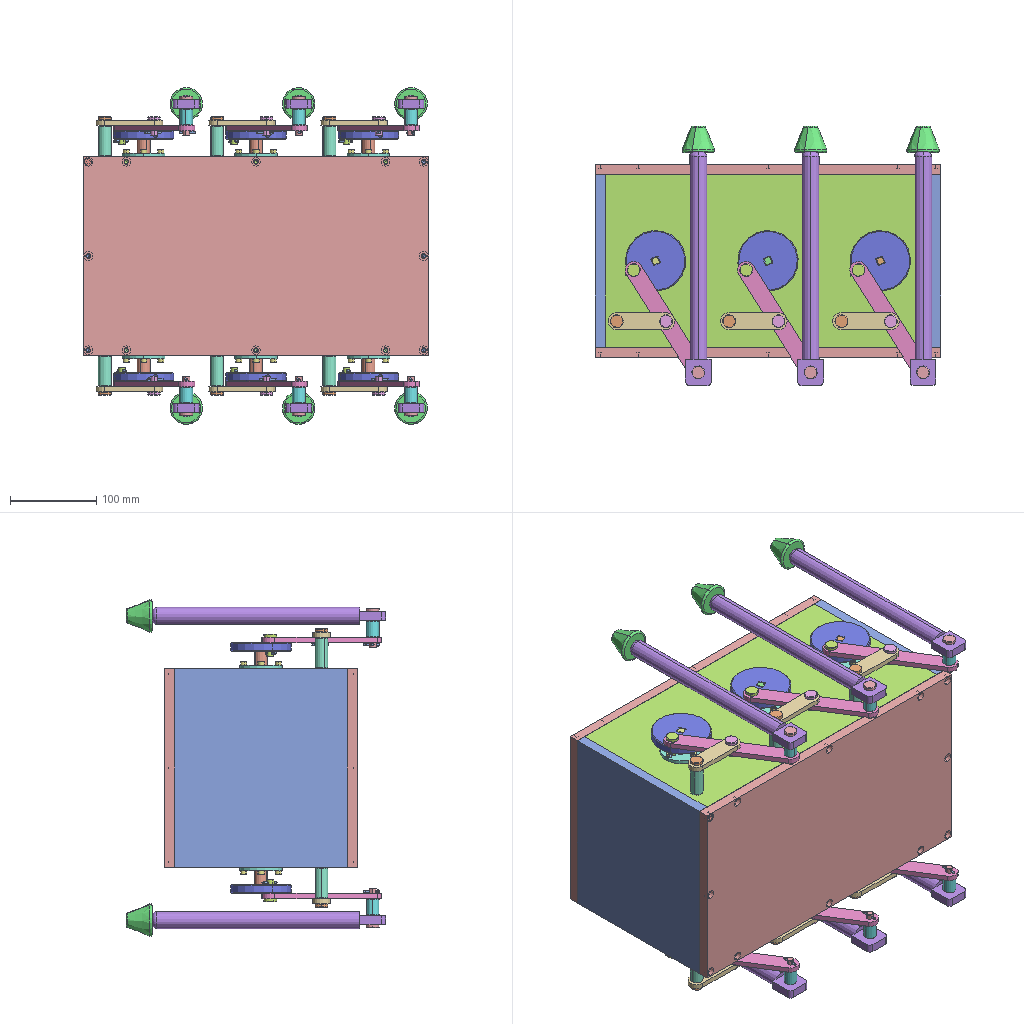Assembly | SolidWorks | 34 different items | 170 placed | box 400 x 300 x 390 mm
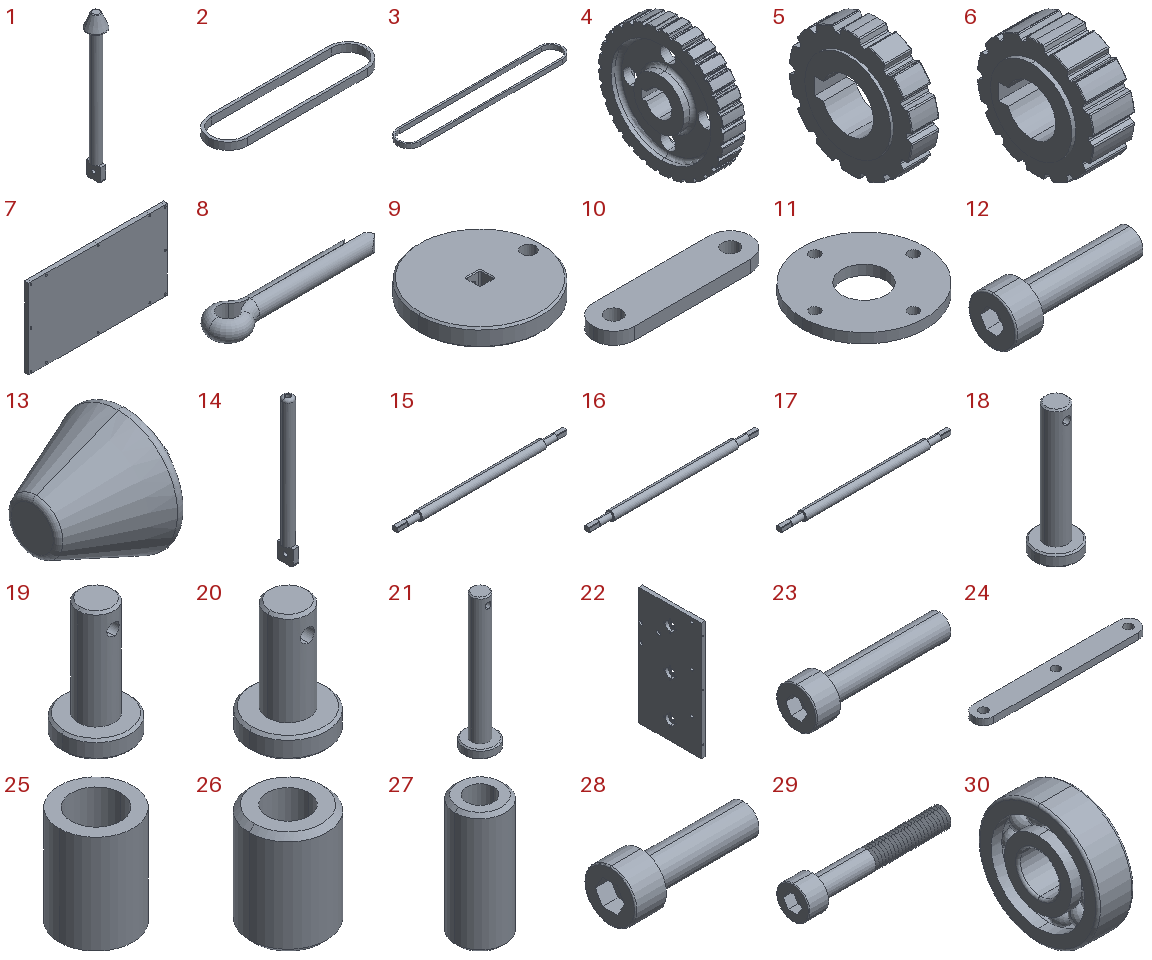Parts list (item | name | quantity | parent item | size | volume | features):
1 | (subassembly) | x6 | - | 38.092 x 38.092 x 300 mm | 102334 mm3 | -
2 | - | x1 | - | 171.8 x 41.8 x 7.9 mm | 9051 mm3 | features Extrusion 1, Shell 1
3 | - | x1 | - | 301.8 x 41.8 x 7.9 mm | 15213 mm3 | features Extrusion 1, Shell 1
4 | - | x1 | - | 15.24 x 72.254 x 72.292 mm | 33206 mm3 | features Cut 3, CirPattern 2, ICE 2, Chamfer 1, Fillet 1, RefAxis 1, Revolution 1
5 | - | x4 | - | 9.48 x 35.738 x 35.892 mm | 6598 mm3 | features ICE 3, Cut 2, Chamfer 1, CirPattern 1, Fillet 1, RefAxis 1, Revolution 1
6 | - | x1 | - | 15.24 x 35.738 x 35.892 mm | 10593 mm3 | features ICE 3, Cut 2, Chamfer 1, CirPattern 1, Fillet 1, RefAxis 1, Revolution 1
7 | - | x2 | - | 400 x 12 x 230 mm | 1097029 mm3 | features Extrusion 1, HoleWzd 1
8 | - | x24 | - | 19.5 x 4.6 x 2.3 mm | 75.866 mm3 | features ICE 1, Sweep 1
9 | - | x6 | - | 70 x 70 x 10 mm | 36483 mm3 | features ICE 4, Chamfer 2, 3DProfileFeature 1, Cut 1, Extrusion 1, Fillet 1, HoleWzd 1
10 | - | x6 | - | 77.02 x 20 x 6 mm | 8124 mm3 | features Extrusion 1, ICE 1
11 | - | x6 | - | 50 x 50 x 4 mm | 6614 mm3 | features Extrusion 1
12 | - | x24 | - | 20 x 7 x 7 mm | 339.552 mm3 | features BlendCut 1, Cut 1, Fillet 1, LPattern 1, RevCut 1, Revolution 1
13 | - | x6 | in 1 | 40 x 38.092 x 38.092 mm | 19850 mm3 | features Fillet 2, ICE 1, Revolution 1
14 | - | x6 | in 1 | 20 x 30 x 270 mm | 82484 mm3 | features ICE 3, Fillet 2, Extrusion 1
15 | - | x1 | - | 290 x 17.22 x 15 mm | 43056 mm3 | features ICE 3, Chamfer 1, Cut 1, Extrusion 1, Fillet 1, MirrorPattern 1
16 | - | x1 | - | 290 x 17.22 x 15 mm | 43172 mm3 | features ICE 3, Chamfer 1, Cut 1, Extrusion 1, Fillet 1, MirrorPattern 1
17 | - | x1 | - | 290 x 15 x 17.22 mm | 43129 mm3 | features ICE 3, Chamfer 1, Cut 1, Extrusion 1, Fillet 1, MirrorPattern 1
18 | - | x6 | - | 15 x 15 x 46 mm | 2758 mm3 | features ICE 2, Chamfer 1, Extrusion 1
19 | - | x6 | - | 15 x 15 x 26 mm | 1753 mm3 | features ICE 2, Chamfer 1, Extrusion 1
20 | - | x6 | - | 15 x 15 x 22 mm | 1552 mm3 | features ICE 2, Chamfer 1, Extrusion 1
21 | - | x6 | - | 15 x 15 x 64 mm | 3663 mm3 | features ICE 2, Chamfer 1, Extrusion 1
22 | - | x1 | - | 12 x 200 x 376 mm | 873388 mm3 | features HoleWzd 1, MirrorStock 1
23 | - | x2 | - | 30 x 8.5 x 8.5 mm | 740.448 mm3 | features BlendCut 1, Cut 1, Fillet 1, LPattern 1, RevCut 1, Revolution 1
24 | - | x6 | - | 160 x 20 x 6 mm | 17780 mm3 | features ICE 2, Extrusion 1
25 | - | x6 | - | 15 x 15 x 20 mm | 1963 mm3 | features Extrusion 1
26 | - | x6 | - | 15 x 15 x 20 mm | 2484 mm3 | features Chamfer 1, Extrusion 1, ICE 1
27 | - | x6 | - | 15 x 15 x 36 mm | 4507 mm3 | features Chamfer 1, Extrusion 1, ICE 1
28 | - | x3 | - | 26 x 10 x 10 mm | 972.813 mm3 | features BlendCut 1, Cut 1, Fillet 1, LPattern 1, RevCut 1, Revolution 1
29 | - | x3 | - | 46 x 10 x 10 mm | 1365 mm3 | features BlendCut 1, Cut 1, Fillet 1, LPattern 1, RevCut 1, Revolution 1
30 | - | x6 | - | 9 x 30 x 30 mm | 4205 mm3 | features Revolution 3, CirPattern 1, Fillet 1
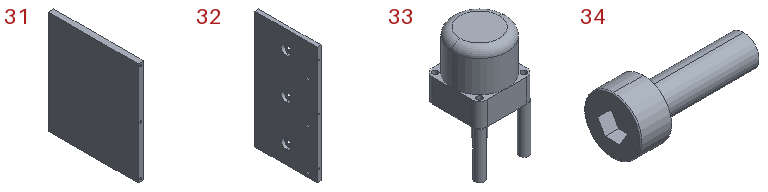31 | - | x2 | - | 12 x 200 x 230 mm | 549928 mm3 | features Extrusion 1, HoleWzd 1, MirrorPattern 1
32 | - | x1 | - | 12 x 200 x 376 mm | 876393 mm3 | features Cut 2, HoleWzd 2, Extrusion 1, ICE 1, MirrorPattern 1
33 | - | x1 | - | 70 x 70 x 140 mm | 361948 mm3 | features Chamfer 5, ICE 5, Fillet 2, HoleWzd 2, CirPattern 1, Extrusion 1
34 | - | x6 | - | 13 x 5.5 x 5.5 mm | 134.528 mm3 | features BlendCut 1, Cut 1, Fillet 1, LPattern 1, RevCut 1, Revolution 1
Mates (type | each side: item.copy, entity, surface, feature):
In the top assembly
Concentric | 7.1 face cylinder CBORE for M5 Hex Socket Head Cap Screw1 | 31.1 face cylinder M5 Tapped Hole1 | 2 times
Coincident | 7.1 face plane Boss-Extrude1 | 31.1 face plane Boss-Extrude1
Concentric | 7.1 face cylinder CBORE for M5 Hex Socket Head Cap Screw1 | 31.2 edge
Concentric | 7.1 face cylinder CBORE for M5 Hex Socket Head Cap Screw1 | 31.2 face cylinder M5 Tapped Hole1
Coincident | 7.1 face plane Boss-Extrude1 | 31.2 face plane Boss-Extrude1
Concentric | 7.1 face cylinder CBORE for M5 Hex Socket Head Cap Screw1 | 32.1 face cylinder Mirror1 | 2 times
Coincident | 7.1 face plane Boss-Extrude1 | 32.1 face plane Boss-Extrude1
Concentric | 31.1 face cylinder Mirror1 | 7.2 face cylinder CBORE for M5 Hex Socket Head Cap Screw1
Concentric | 32.1 face cylinder Mirror1 | 7.2 face cylinder CBORE for M5 Hex Socket Head Cap Screw1
Coincident | 31.1 face plane Boss-Extrude1 | 7.2 face plane Boss-Extrude1
Concentric | 32.1 face cylinder Cut-Extrude1 | 30.1 face cylinder Revolve3
Coincident | 32.1 face plane Boss-Extrude1 | 30.1 face plane Revolve3
Concentric | 32.1 face cylinder Cut-Extrude1 | 30.2 face cylinder Revolve3
Coincident | 32.1 face plane Boss-Extrude1 | 30.2 face plane Revolve3
Concentric | 32.1 face cylinder Cut-Extrude1 | 30.3 face cylinder Revolve3
Coincident | 32.1 face plane Boss-Extrude1 | 30.3 face plane Revolve3
Concentric | 30.4 face cylinder Revolve2 | 11.1 face cylinder Boss-Extrude1
Concentric | 30.3 face cylinder Revolve2 | 11.2 face cylinder Boss-Extrude1
Coincident | 32.1 face plane Boss-Extrude1 | 11.2 face plane Boss-Extrude1
Concentric | 30.1 face cylinder Revolve2 | 15.1 face cylinder Boss-Extrude1
Coincident | 30.1 face plane Revolve2 | 15.1 face plane Boss-Extrude1
Concentric | 30.2 face cylinder Revolve2 | 16.1 face cylinder Boss-Extrude1
Coincident | 30.2 face plane Revolve2 | 16.1 face plane Boss-Extrude1
Concentric | 30.3 face cylinder Revolve2 | 17.1 face cylinder Boss-Extrude1
Coincident | 30.3 face plane Revolve2 | 17.1 face plane Boss-Extrude1
Concentric | 17.1 face cylinder Boss-Extrude2 | 25.1 face cylinder Boss-Extrude1
Coincident | 30.4 face plane Revolve2 | 25.1 face plane Boss-Extrude1
Concentric | 17.1 face cylinder Boss-Extrude2 | 25.2 face cylinder Boss-Extrude1
Coincident | 30.3 face plane Revolve2 | 25.2 face plane Boss-Extrude1
Coincident | 17.1 face plane Cut-Extrude1 | 9.1 face plane Cut-Extrude3 | 2 times
Coincident | 25.1 face plane Boss-Extrude1 | 9.1 face plane Boss-Extrude1
Coincident | 16.1 face plane Mirror1 | 9.2 face plane Cut-Extrude3 | 2 times
Coincident | 25.3 face plane Boss-Extrude1 | 9.2 face plane Boss-Extrude1
Coincident | 15.1 face plane Cut-Extrude1 | 9.3 face plane Cut-Extrude3 | 2 times
Coincident | 25.4 face plane Boss-Extrude1 | 9.3 face plane Boss-Extrude1
Coincident | 17.1 face plane Mirror1 | 9.4 face plane Cut-Extrude3 | 2 times
Coincident | 25.2 face plane Boss-Extrude1 | 9.4 face plane Boss-Extrude1
Coincident | 16.1 face plane Cut-Extrude1 | 9.5 face plane Cut-Extrude3 | 2 times
Coincident | 25.5 face plane Boss-Extrude1 | 9.5 face plane Boss-Extrude1
Coincident | 15.1 face plane Mirror1 | 9.6 face plane Cut-Extrude3 | 2 times
Coincident | 25.6 face plane Boss-Extrude1 | 9.6 face plane Boss-Extrude1
Concentric | 9.6 face cylinder Cut-Extrude2 | 24.1 face cylinder Cut-Extrude1
Coincident | 9.6 face plane Boss-Extrude1 | 24.1 face plane Boss-Extrude1
Concentric | 9.5 face cylinder Cut-Extrude2 | 24.2 face cylinder Cut-Extrude1
Coincident | 9.5 face plane Boss-Extrude1 | 24.2 face plane Boss-Extrude1
Concentric | 9.4 face cylinder Cut-Extrude2 | 24.3 face cylinder Cut-Extrude1
Coincident | 9.4 face plane Boss-Extrude1 | 24.3 face plane Boss-Extrude1
Concentric | 9.3 face cylinder Cut-Extrude2 | 24.4 face cylinder Cut-Extrude1
Coincident | 9.3 face plane Boss-Extrude1 | 24.4 face plane Boss-Extrude1
Coincident | 9.2 face plane Boss-Extrude1 | 24.5 face plane Boss-Extrude1
Concentric | 9.2 face cylinder Cut-Extrude2 | 24.5 face cylinder Cut-Extrude1
Coincident | 9.1 face plane Boss-Extrude1 | 24.6 face plane Boss-Extrude1
Concentric | 9.1 face cylinder Cut-Extrude2 | 24.6 face cylinder Cut-Extrude1
Coincident | 24.3 face plane Boss-Extrude1 | 26.1 face plane Boss-Extrude1
Concentric | 24.3 face cylinder Cut-Extrude1 | 26.1 face cylinder Boss-Extrude1
Concentric | 24.2 face cylinder Cut-Extrude1 | 26.2 face cylinder Boss-Extrude1
Coincident | 24.2 face plane Boss-Extrude1 | 26.2 face plane Boss-Extrude1
Concentric | 24.1 edge | 26.3 face cylinder Boss-Extrude1
Coincident | 24.1 face plane Boss-Extrude1 | 26.3 face plane Boss-Extrude1
Concentric | 24.4 face cylinder Cut-Extrude1 | 26.4 face cylinder Boss-Extrude1
Coincident | 24.4 face plane Boss-Extrude1 | 26.4 face plane Boss-Extrude1
Concentric | 24.5 face cylinder Cut-Extrude1 | 26.5 face cylinder Boss-Extrude1
Coincident | 24.5 face plane Boss-Extrude1 | 26.5 face plane Boss-Extrude1
Concentric | 24.6 face cylinder Cut-Extrude1 | 26.6 face cylinder Boss-Extrude1
Coincident | 24.6 face plane Boss-Extrude1 | 26.6 face plane Boss-Extrude1
Concentric | 24.1 face cylinder Cut-Extrude2 | 10.1 face cylinder Cut-Extrude1
Coincident | 24.1 face plane Boss-Extrude1 | 10.1 face plane Boss-Extrude1
Coincident | 24.2 face plane Boss-Extrude1 | 10.2 face plane Boss-Extrude1
Concentric | 24.2 face cylinder Cut-Extrude2 | 10.2 face cylinder Cut-Extrude1
Coincident | 24.3 face plane Boss-Extrude1 | 10.3 face plane Boss-Extrude1
Concentric | 24.3 face cylinder Cut-Extrude2 | 10.3 face cylinder Cut-Extrude1
Coincident | 24.5 face plane Boss-Extrude1 | 10.4 face plane Boss-Extrude1
Concentric | 24.5 face cylinder Cut-Extrude2 | 10.4 face cylinder Cut-Extrude1
Coincident | 24.4 face plane Boss-Extrude1 | 10.5 face plane Boss-Extrude1
Concentric | 24.4 face cylinder Cut-Extrude2 | 10.5 face cylinder Cut-Extrude1
Concentric | 26.4 face cylinder Boss-Extrude1 | 14.1 face cylinder Cut-Extrude1
Coincident | 26.4 face plane Boss-Extrude1 | 14.1 face plane Boss-Extrude2
Concentric | 26.5 face cylinder Boss-Extrude1 | 14.2 face cylinder Cut-Extrude1
Coincident | 26.5 face plane Boss-Extrude1 | 14.2 face plane Boss-Extrude2
Concentric | 26.6 face cylinder Boss-Extrude1 | 14.3 face cylinder Cut-Extrude1
Coincident | 26.6 face plane Boss-Extrude1 | 14.3 face plane Boss-Extrude2
Concentric | 32.1 face cylinder Cut-Extrude3 | 10.1 face cylinder Cut-Extrude1
Concentric | 32.1 face cylinder Cut-Extrude3 | 10.2 face cylinder Cut-Extrude1
Concentric | 32.1 face cylinder Cut-Extrude3 | 10.3 face cylinder Cut-Extrude1
Coincident | 24.6 face plane Boss-Extrude1 | 10.6 face plane Boss-Extrude1
Concentric | 24.6 face cylinder Cut-Extrude2 | 10.6 face cylinder Cut-Extrude1
Concentric | 22.1 face cylinder Side Plate2 Mirror | 10.6 face cylinder Cut-Extrude1
Concentric | 22.1 face cylinder Side Plate2 Mirror | 10.4 face cylinder Cut-Extrude1
Concentric | 22.1 face cylinder Side Plate2 Mirror | 10.5 face cylinder Cut-Extrude1
Concentric | 26.3 face cylinder Boss-Extrude1 | 14.4 face cylinder Cut-Extrude1
Coincident | 26.3 face plane Boss-Extrude1 | 14.4 face plane Boss-Extrude2
Concentric | 26.2 face cylinder Boss-Extrude1 | 14.5 face cylinder Cut-Extrude1
Coincident | 26.2 face plane Boss-Extrude1 | 14.5 face plane Boss-Extrude2
Concentric | 26.1 face cylinder Boss-Extrude1 | 14.6 face cylinder Cut-Extrude1
Coincident | 26.1 face plane Boss-Extrude1 | 14.6 face plane Boss-Extrude2
Coincident | 10.3 face plane Boss-Extrude1 | 10.2 face plane Boss-Extrude1
Coincident | 10.2 face plane Boss-Extrude1 | 10.1 face plane Boss-Extrude1
Concentric | 18.1 face cylinder Boss-Extrude1 | 24.4 face cylinder Cut-Extrude1
Coincident | 14.1 face plane Boss-Extrude2 | 18.1 face plane Boss-Extrude2
Concentric | 14.2 face cylinder Cut-Extrude1 | 18.2 face cylinder Boss-Extrude1
Coincident | 14.2 face plane Boss-Extrude2 | 18.2 face plane Boss-Extrude2
Concentric | 14.3 face cylinder Cut-Extrude1 | 18.3 face cylinder Boss-Extrude1
Coincident | 14.3 face plane Boss-Extrude2 | 18.3 face plane Boss-Extrude2
Coincident | 14.4 edge | 18.4 face cylinder Boss-Extrude1
Coincident | 14.4 face plane Boss-Extrude2 | 18.4 face plane Boss-Extrude2
Concentric | 14.5 face cylinder Cut-Extrude1 | 18.5 face cylinder Boss-Extrude1
Coincident | 14.5 face plane Boss-Extrude2 | 18.5 face plane Boss-Extrude2
Coincident | 14.6 edge | 18.6 face cylinder Boss-Extrude1
Coincident | 14.6 face plane Boss-Extrude2 | 18.6 face plane Boss-Extrude2
Concentric | 18.6 face cylinder Cut-Extrude1 | 8.1 face cylinder Sweep2
DistanceDim | 8.1 plane | 26.1 plane
Concentric | 18.5 face cylinder Cut-Extrude1 | 8.2 face cylinder Sweep2
DistanceDim | 8.2 plane | 26.2 plane
Concentric | 18.4 face cylinder Cut-Extrude1 | 8.3 face cylinder Sweep2
DistanceDim | 8.3 plane | 26.3 plane
Concentric | 18.3 face cylinder Cut-Extrude1 | 8.4 face cylinder Sweep2
DistanceDim | 8.4 plane | 26.6 plane
Concentric | 18.2 face cylinder Cut-Extrude1 | 8.5 face cylinder Sweep2
DistanceDim | 8.5 plane | 26.5 plane
Concentric | 18.1 face cylinder Cut-Extrude1 | 8.6 face cylinder Sweep2
DistanceDim | 8.6 plane | 26.4 plane
Concentric | 24.1 face cylinder Cut-Extrude1 | 19.1 face cylinder Boss-Extrude1
Coincident | 24.1 face plane Boss-Extrude1 | 19.1 face plane Boss-Extrude2
Concentric | 24.2 face cylinder Cut-Extrude1 | 19.2 face cylinder Boss-Extrude1
Coincident | 24.2 face plane Boss-Extrude1 | 19.2 face plane Boss-Extrude2
Concentric | 24.3 face cylinder Cut-Extrude1 | 19.3 face cylinder Boss-Extrude1
Coincident | 24.3 face plane Boss-Extrude1 | 19.3 face plane Boss-Extrude2
Concentric | 24.6 face cylinder Cut-Extrude1 | 19.4 face cylinder Boss-Extrude1
Coincident | 24.6 face plane Boss-Extrude1 | 19.4 face plane Boss-Extrude2
Concentric | 24.5 face cylinder Cut-Extrude1 | 19.5 face cylinder Boss-Extrude1
Coincident | 24.5 face plane Boss-Extrude1 | 19.5 face plane Boss-Extrude2
Concentric | 24.4 face cylinder Cut-Extrude1 | 19.6 face cylinder Boss-Extrude1
Coincident | 24.4 face plane Boss-Extrude1 | 19.6 face plane Boss-Extrude2
Concentric | 19.6 face cylinder Cut-Extrude1 | 8.7 face cylinder Sweep2
DistanceDim | 8.7 plane | 9.3 plane
Concentric | 19.5 face cylinder Cut-Extrude1 | 8.8 face cylinder Sweep2
DistanceDim | 8.8 plane | 9.2 plane
Concentric | 19.4 face cylinder Cut-Extrude1 | 8.9 face cylinder Sweep2
DistanceDim | 8.9 plane | 24.6 plane
Concentric | 19.1 face cylinder Cut-Extrude1 | 8.10 face cylinder Sweep2
Concentric | 19.2 face cylinder Cut-Extrude1 | 8.11 face cylinder Sweep2
DistanceDim | 8.11 plane | 24.2 plane
Concentric | 19.3 face cylinder Cut-Extrude1 | 8.12 face cylinder Sweep2
DistanceDim | 8.12 plane | 24.3 plane
Concentric | 10.5 face cylinder Cut-Extrude1 | 20.1 face cylinder Boss-Extrude1
Coincident | 10.5 face plane Boss-Extrude1 | 20.1 face plane Boss-Extrude2
Concentric | 10.4 face cylinder Cut-Extrude1 | 20.2 face cylinder Boss-Extrude1
Coincident | 10.4 face plane Boss-Extrude1 | 20.2 face plane Boss-Extrude2
Concentric | 10.6 face cylinder Cut-Extrude1 | 20.3 face cylinder Boss-Extrude1
Coincident | 10.6 face plane Boss-Extrude1 | 20.3 face plane Boss-Extrude2
Concentric | 10.3 face cylinder Cut-Extrude1 | 20.4 face cylinder Boss-Extrude1
Coincident | 10.3 face plane Boss-Extrude1 | 20.4 face plane Boss-Extrude2
Concentric | 10.2 face cylinder Cut-Extrude1 | 20.5 face cylinder Boss-Extrude1
Coincident | 10.2 face plane Boss-Extrude1 | 20.5 face plane Boss-Extrude2
Concentric | 10.1 face cylinder Cut-Extrude1 | 20.6 face cylinder Boss-Extrude1
Coincident | 10.1 face plane Boss-Extrude1 | 20.6 face plane Boss-Extrude2
Concentric | 20.6 face cylinder Cut-Extrude1 | 8.13 face cylinder Sweep2
DistanceDim | 8.13 plane | 10.1 plane
Concentric | 20.5 face cylinder Cut-Extrude1 | 8.14 face cylinder Sweep2
DistanceDim | 8.14 plane | 10.2 plane
Concentric | 20.4 face cylinder Cut-Extrude1 | 8.15 face cylinder Sweep2
DistanceDim | 8.15 plane | 10.3 plane
Concentric | 20.3 face cylinder Cut-Extrude1 | 8.16 face cylinder Sweep2
DistanceDim | 8.16 plane | 10.6 plane
Concentric | 20.2 face cylinder Cut-Extrude1 | 8.17 face cylinder Sweep2
DistanceDim | 8.17 plane | 10.4 plane
Concentric | 20.1 face cylinder Cut-Extrude1 | 8.18 face cylinder Sweep2
DistanceDim | 8.18 plane | 10.5 plane
Concentric | 32.1 face cylinder Cut-Extrude3 | 27.1 face cylinder Boss-Extrude1
Coincident | 32.1 face plane Boss-Extrude1 | 27.1 face plane Boss-Extrude1
Concentric | 32.1 face cylinder Cut-Extrude3 | 27.2 face cylinder Boss-Extrude1
Coincident | 32.1 face plane Boss-Extrude1 | 27.2 face plane Boss-Extrude1
Concentric | 32.1 face cylinder Cut-Extrude3 | 27.3 face cylinder Boss-Extrude1
Coincident | 32.1 face plane Boss-Extrude1 | 27.3 face plane Boss-Extrude1
Concentric | 22.1 face cylinder Side Plate2 Mirror | 27.4 face cylinder Boss-Extrude1
Coincident | 22.1 face plane Side Plate2 Mirror | 27.4 face plane Boss-Extrude1
Concentric | 22.1 face cylinder Side Plate2 Mirror | 27.5 face cylinder Boss-Extrude1
Coincident | 22.1 face plane Side Plate2 Mirror | 27.5 face plane Boss-Extrude1
Concentric | 22.1 face cylinder Side Plate2 Mirror | 27.6 face cylinder Boss-Extrude1
Coincident | 22.1 face plane Side Plate2 Mirror | 27.6 face plane Boss-Extrude1
Concentric | 10.5 face cylinder Cut-Extrude1 | 21.1 face cylinder Boss-Extrude1
Coincident | 10.5 face plane Boss-Extrude1 | 21.1 face plane Boss-Extrude2
Concentric | 10.4 face cylinder Cut-Extrude1 | 21.2 face cylinder Boss-Extrude1
Coincident | 10.4 face plane Boss-Extrude1 | 21.2 face plane Boss-Extrude2
Concentric | 10.6 face cylinder Cut-Extrude1 | 21.3 face cylinder Boss-Extrude1
Coincident | 10.6 face plane Boss-Extrude1 | 21.3 face plane Boss-Extrude2
Concentric | 10.3 face cylinder Cut-Extrude1 | 21.4 face cylinder Boss-Extrude1
Coincident | 10.3 face plane Boss-Extrude1 | 21.4 face plane Boss-Extrude2
Concentric | 10.2 face cylinder Cut-Extrude1 | 21.5 face cylinder Boss-Extrude1
Coincident | 10.2 face plane Boss-Extrude1 | 21.5 face plane Boss-Extrude2
Concentric | 10.1 face cylinder Cut-Extrude1 | 21.6 face cylinder Boss-Extrude1
Coincident | 10.1 face plane Boss-Extrude1 | 21.6 face plane Boss-Extrude2
Concentric | 21.4 face cylinder Cut-Extrude1 | 8.19 face cylinder Sweep2
DistanceDim | 8.19 plane | 27.1 plane
Concentric | 21.5 face cylinder Cut-Extrude1 | 8.20 face cylinder Sweep2
DistanceDim | 8.20 plane | 27.2 plane
Concentric | 21.6 face cylinder Cut-Extrude1 | 8.21 face cylinder Sweep2
DistanceDim | 8.21 plane | 27.3 plane
Concentric | 21.3 face cylinder Cut-Extrude1 | 8.22 face cylinder Sweep2
DistanceDim | 8.22 plane | 27.4 plane
Concentric | 21.2 face cylinder Cut-Extrude1 | 8.23 face cylinder Sweep2
DistanceDim | 8.23 plane | 27.5 plane
Concentric | 21.1 face cylinder Cut-Extrude1 | 8.24 face cylinder Sweep2
DistanceDim | 8.24 plane | 27.6 plane
Parallel | 14.1 face plane Boss-Extrude2 | 14.2 face plane Boss-Extrude2
Parallel | 14.2 face plane Boss-Extrude2 | 14.3 face plane Boss-Extrude2
Parallel | 14.1 face plane Boss-Extrude2 | 14.4 face plane Boss-Extrude2
Parallel | 14.4 face plane Boss-Extrude2 | 14.5 face plane Boss-Extrude2
Parallel | 14.5 face plane Boss-Extrude2 | 14.6 face plane Boss-Extrude2
Parallel | 31.2 face plane Boss-Extrude1 | 14.1 face plane Boss-Extrude2
Coincident | 7.1 face plane Boss-Extrude1 | 33.1 face plane Boss-Extrude1
DistanceDim | 33.1 face plane Boss-Extrude1 | 31.1 face plane Boss-Extrude1
Coincident | 22.1 face plane Side Plate2 Mirror | 33.1 face plane Boss-Extrude6
DistanceDim | 8.10 plane | 24.1 plane
Concentric | 11.3 face cylinder Boss-Extrude1 | 12.1 face cylinder Base-Revolve
Coincident | 11.3 face plane Boss-Extrude1 | 12.1 face plane Base-Revolve
Concentric | 32.1 face cylinder M4 Tapped Hole1 | 11.3 face cylinder Boss-Extrude1
Concentric | 32.1 face cylinder M4 Tapped Hole1 | 11.4 face cylinder Boss-Extrude1
Concentric | 32.1 face cylinder M4 Tapped Hole1 | 11.2 face cylinder Boss-Extrude1
Concentric | 11.1 face cylinder Boss-Extrude1 | 22.1 face cylinder Side Plate2 Mirror
Concentric | 11.5 face cylinder Boss-Extrude1 | 22.1 face cylinder Side Plate2 Mirror
Concentric | 11.6 face cylinder Boss-Extrude1 | 22.1 face cylinder Side Plate2 Mirror
Concentric | 11.6 face cylinder Boss-Extrude1 | 12.2 face cylinder Base-Revolve
Coincident | 11.6 face plane Boss-Extrude1 | 12.2 face plane Base-Revolve
Concentric | 22.1 face cylinder CBORE for M6 Hex Head Bolt1 | 28.1 face cylinder Base-Revolve
Coincident | 22.1 face plane CBORE for M6 Hex Head Bolt1 | 28.1 face plane Base-Revolve
Concentric | 22.1 face cylinder CBORE for M6 Hex Head Bolt1 | 28.2 face cylinder Base-Revolve
Coincident | 22.1 face plane CBORE for M6 Hex Head Bolt1 | 28.2 face plane Base-Revolve
Concentric | 22.1 face cylinder CBORE for M6 Hex Head Bolt1 | 28.3 face cylinder Base-Revolve
Coincident | 22.1 face plane CBORE for M6 Hex Head Bolt1 | 28.3 face plane Base-Revolve
Concentric | 33.1 face cylinder CirPattern1 | 29.1 face cylinder Base-Revolve
Coincident | 33.1 face plane Boss-Extrude1 | 29.1 face plane Base-Revolve
Concentric | 33.1 face cylinder CirPattern1 | 29.2 face cylinder Base-Revolve
Coincident | 33.1 face plane Boss-Extrude1 | 29.2 face plane Base-Revolve
Concentric | 33.1 face cylinder CirPattern1 | 29.3 face cylinder Base-Revolve
Coincident | 33.1 face plane Boss-Extrude1 | 29.3 face plane Base-Revolve
Concentric | 7.2 face cylinder CBORE for M5 Hex Socket Head Cap Screw1 | 23.1 face cylinder Base-Revolve
Coincident | 7.2 face plane CBORE for M5 Hex Socket Head Cap Screw1 | 23.1 face plane Base-Revolve
Concentric | 7.1 face cylinder CBORE for M5 Hex Socket Head Cap Screw1 | 23.2 face cylinder Base-Revolve
Coincident | 7.1 face plane CBORE for M5 Hex Socket Head Cap Screw1 | 23.2 face plane Base-Revolve
Concentric | 9.6 face cylinder Cut-Extrude5 | 34.1 face cylinder Base-Revolve
Coincident | 9.6 face plane Cut-Extrude5 | 34.1 face plane Base-Revolve
Concentric | 9.5 face cylinder Cut-Extrude5 | 34.2 face cylinder Base-Revolve
Coincident | 9.5 face plane Cut-Extrude5 | 34.2 face plane Base-Revolve
Concentric | 9.4 face cylinder Cut-Extrude5 | 34.3 face cylinder Base-Revolve
Coincident | 9.4 face plane Cut-Extrude5 | 34.3 face plane Base-Revolve
Concentric | 9.3 face cylinder Cut-Extrude5 | 34.4 face cylinder Base-Revolve
Coincident | 9.3 face plane Cut-Extrude5 | 34.4 face plane Base-Revolve
Coincident | 9.2 face plane Cut-Extrude5 | 34.5 face plane Base-Revolve
Concentric | 9.2 face cylinder Cut-Extrude5 | 34.5 face cylinder Base-Revolve
Coincident | 9.1 face plane Cut-Extrude5 | 34.6 face plane Base-Revolve
Concentric | 9.1 face cylinder Cut-Extrude5 | 34.6 face cylinder Base-Revolve
Concentric | 33.1 face cylinder Boss-Extrude4 | 6.1 face cylinder Cut-Extrude4
DistanceDim | 6.1 face plane Revolve1 | 33.1 face plane Boss-Extrude4
Parallel | 7.1 face plane Boss-Extrude1 | 6.1 face plane Cut-Extrude4
Concentric | 16.1 face cylinder Boss-Extrude1 | 4.1 face cylinder Cut-Extrude5
Coincident | 6.1 face plane Revolve1 | 4.1 face plane Revolve1
Parallel | 7.1 face plane Boss-Extrude1 | 4.1 face plane Cut-Extrude5
Concentric | 16.1 face cylinder Boss-Extrude1 | 5.1 face cylinder Cut-Extrude4
DistanceDim | 5.1 face plane Revolve1 | 4.1 face plane Revolve1
Parallel | 4.1 face plane Cut-Extrude5 | 5.1 face plane Cut-Extrude4
Concentric | 17.1 face cylinder Boss-Extrude1 | 5.2 face cylinder Cut-Extrude4
Coincident | 5.1 face plane Revolve1 | 5.2 face plane Revolve1
Coincident | 5.1 face plane Cut-Extrude4 | 5.2 face plane Cut-Extrude4
Concentric | 17.1 face cylinder Boss-Extrude1 | 5.3 face cylinder Cut-Extrude4
DistanceDim | 5.3 face plane Revolve1 | 5.2 face plane Revolve1
Coincident | 5.3 face plane Cut-Extrude4 | 5.2 face plane Cut-Extrude4
Concentric | 15.1 face cylinder Boss-Extrude1 | 5.4 face cylinder Cut-Extrude4
Coincident | 5.4 face plane Revolve1 | 5.3 face plane Revolve1
Coincident | 5.4 face plane Cut-Extrude4 | 5.3 face plane Cut-Extrude4
Concentric | 5.1 face cylinder Revolve1 | 2.1 face cylinder Shell1
Concentric | 5.2 face cylinder Revolve1 | 2.1 face cylinder Shell1
Coincident | 5.2 face plane Revolve1 | 2.1 face plane Boss-Extrude1
Concentric | 5.3 face cylinder Revolve1 | 3.1 face cylinder Shell1
Concentric | 5.4 face cylinder Revolve1 | 3.1 face cylinder Shell1
Coincident | 5.3 face plane Revolve1 | 3.1 face plane Boss-Extrude1
In subassembly 1
Concentric | 14.7 face cylinder Cut-Extrude2 | 13.1 face cylinder Boss-Extrude1
Coincident | 14.7 face plane Boss-Extrude1 | 13.1 face plane Revolve1